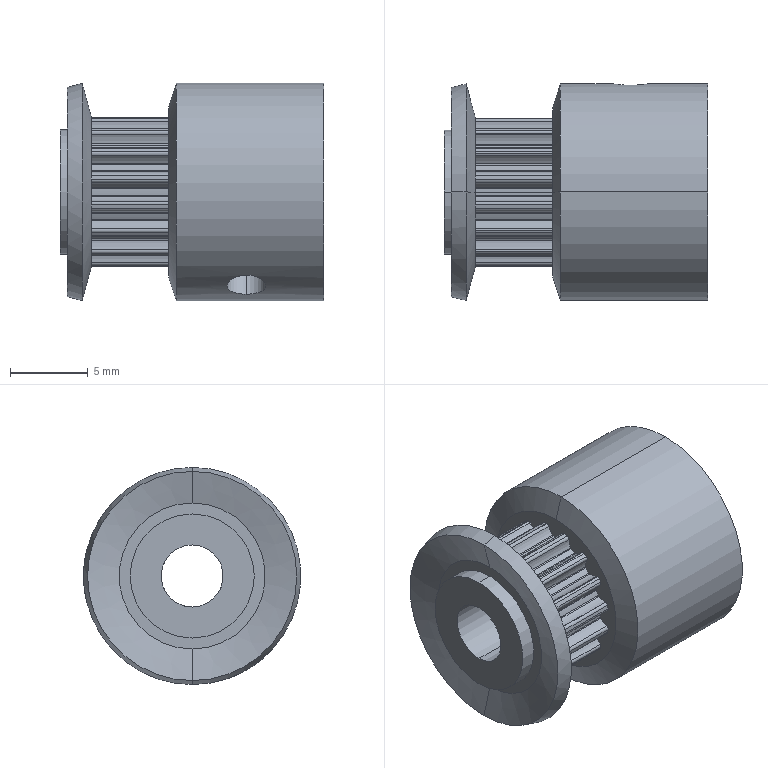Part | SolidWorks | 3 solids | 227 faces | box 17 x 14 x 14 mm | volume 1805 mm3 | cylinder 159 | plane 48 | cone 20 | commonest cylinder face diameters 0.38 x40 0.2 x36 2.65 x36 8.16 x17 9.68 x16 2.459 x4